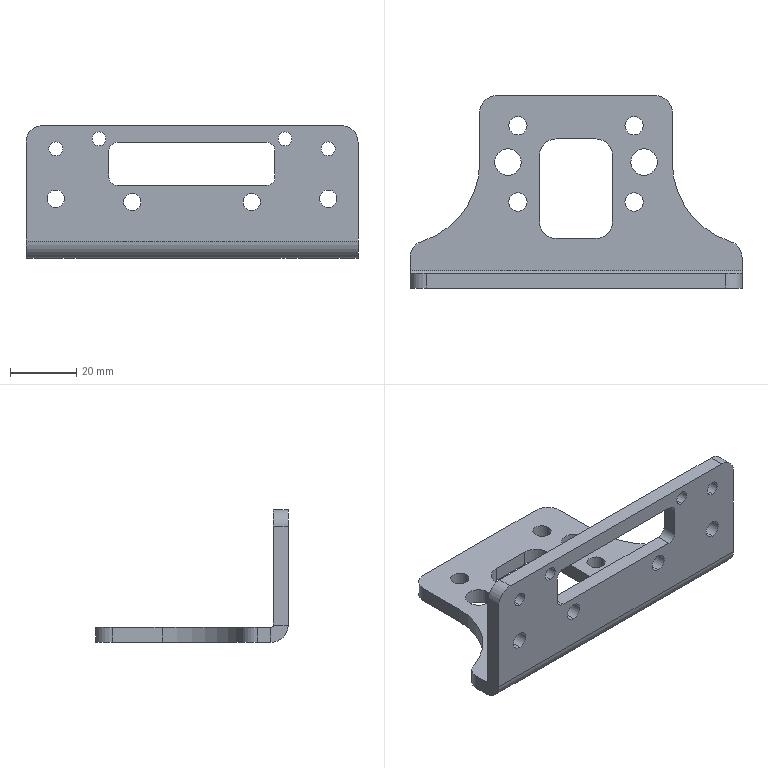Part | STEP file | 1 solid | 68 faces | box 100 x 58 x 40 mm | volume 26779 mm3 | cylinder 46 | plane 22 | commonest cylinder face diameters 10 x10 4.2 x8 5.2 x8 5.5 x8 5 x4 8 x4